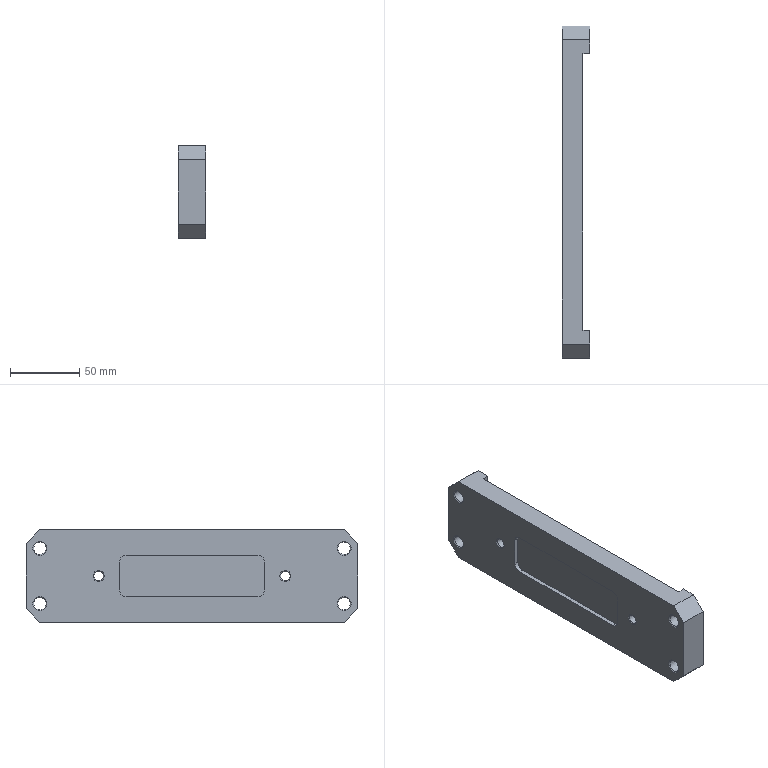Part | NX | features DATUM_CSYS 6, SIMPLE HOLE 6, SKETCH 5, EXTRUDE 3, HOLE PACKAGE 2, LINKED_CURVE 2, SYMBOLIC_THREAD 2, BLEND 1, CHAMFER 1, LINKED_FACE 1 | 1 solid | 41 faces | box 20 x 240 x 67 mm | volume 234977 mm3 | plane 19 | cone 12 | cylinder 10 | commonest cylinder face diameters 9 x4 10 x4 6.8 x2
STEP:
#1=CARTESIAN_POINT('',(65.,-120.,-393.));
#2=VERTEX_POINT('',#1);
#3=CARTESIAN_POINT('',(65.,-120.,-440.));
#4=VERTEX_POINT('',#3);
#5=CARTESIAN_POINT('',(65.,-120.,-383.));
#6=DIRECTION('',(0.,0.,-1.));
#7=VECTOR('',#6,1000.);
#8=LINE('',#5,#7);
#9=EDGE_CURVE('',#2,#4,#8,.T.);
#10=ORIENTED_EDGE('',*,*,#9,.F.);
#11=CARTESIAN_POINT('',(65.,-110.,-383.));
#12=VERTEX_POINT('',#11);
#13=CARTESIAN_POINT('',(65.,-120.,-393.));
#14=DIRECTION('',(0.,-0.7071,-0.7071));
#15=VECTOR('',#14,1000.);
#16=LINE('',#13,#15);
#17=EDGE_CURVE('',#2,#12,#16,.F.);
#18=ORIENTED_EDGE('',*,*,#17,.T.);
#19=CARTESIAN_POINT('',(65.,110.,-383.));
#20=VERTEX_POINT('',#19);
#21=CARTESIAN_POINT('',(65.,120.,-383.));
#22=DIRECTION('',(0.,-1.,0.));
#23=VECTOR('',#22,1000.);
#24=LINE('',#21,#23);
#25=EDGE_CURVE('',#20,#12,#24,.T.);
#26=ORIENTED_EDGE('',*,*,#25,.F.);
#27=CARTESIAN_POINT('',(65.,120.,-393.));
#28=VERTEX_POINT('',#27);
#29=CARTESIAN_POINT('',(65.,110.,-383.));
#30=DIRECTION('',(0.,-0.7071,0.7071));
#31=VECTOR('',#30,1000.);
#32=LINE('',#29,#31);
#33=EDGE_CURVE('',#20,#28,#32,.F.);
#34=ORIENTED_EDGE('',*,*,#33,.T.);
#35=CARTESIAN_POINT('',(65.,120.,-440.));
#36=VERTEX_POINT('',#35);
#37=CARTESIAN_POINT('',(65.,120.,-450.));
#38=DIRECTION('',(0.,0.,1.));
#39=VECTOR('',#38,1000.);
#40=LINE('',#37,#39);
#41=EDGE_CURVE('',#36,#28,#40,.T.);
#42=ORIENTED_EDGE('',*,*,#41,.F.);
#43=CARTESIAN_POINT('',(65.,110.,-450.));
#44=VERTEX_POINT('',#43);
#45=CARTESIAN_POINT('',(65.,120.,-440.));
#46=DIRECTION('',(0.,0.7071,0.7071));
#47=VECTOR('',#46,1000.);
#48=LINE('',#45,#47);
#49=EDGE_CURVE('',#36,#44,#48,.F.);
#50=ORIENTED_EDGE('',*,*,#49,.T.);
#51=CARTESIAN_POINT('',(65.,-110.,-450.));
#52=VERTEX_POINT('',#51);
#53=CARTESIAN_POINT('',(65.,-120.,-450.));
#54=DIRECTION('',(0.,1.,0.));
#55=VECTOR('',#54,1000.);
#56=LINE('',#53,#55);
#57=EDGE_CURVE('',#52,#44,#56,.T.);
#58=ORIENTED_EDGE('',*,*,#57,.F.);
#59=CARTESIAN_POINT('',(65.,-110.,-450.));
#60=DIRECTION('',(0.,0.7071,-0.7071));
#61=VECTOR('',#60,1000.);
#62=LINE('',#59,#61);
#63=EDGE_CURVE('',#52,#4,#62,.F.);
#64=ORIENTED_EDGE('',*,*,#63,.T.);
#65=EDGE_LOOP('',(#10,#18,#26,#34,#42,#50,#58,#64));
#66=FACE_BOUND('',#65,.T.);
#67=CARTESIAN_POINT('',(65.,-67.5,-420.5));
#68=VERTEX_POINT('',#67);
#69=CARTESIAN_POINT('',(65.,-67.5,-416.5));
#70=DIRECTION('',(1.,0.,0.));
#71=DIRECTION('',(0.,0.,-1.));
#72=AXIS2_PLACEMENT_3D('',#69,#70,#71);
#73=CIRCLE('',#72,4.);
#74=EDGE_CURVE('',#68,#68,#73,.T.);
#75=ORIENTED_EDGE('',*,*,#74,.T.);
#76=EDGE_LOOP('',(#75));
#77=FACE_BOUND('',#76,.T.);
#78=CARTESIAN_POINT('',(65.,67.5,-420.5));
#79=VERTEX_POINT('',#78);
#80=CARTESIAN_POINT('',(65.,67.5,-416.5));
#81=DIRECTION('',(1.,0.,0.));
#82=DIRECTION('',(0.,0.,-1.));
#83=AXIS2_PLACEMENT_3D('',#80,#81,#82);
#84=CIRCLE('',#83,4.);
#85=EDGE_CURVE('',#79,#79,#84,.T.);
#86=ORIENTED_EDGE('',*,*,#85,.T.);
#87=EDGE_LOOP('',(#86));
#88=FACE_BOUND('',#87,.T.);
#89=CARTESIAN_POINT('',(65.,110.,-401.6));
#90=VERTEX_POINT('',#89);
#91=CARTESIAN_POINT('',(65.,110.,-396.5));
#92=DIRECTION('',(1.,0.,0.));
#93=DIRECTION('',(0.,0.,-1.));
#94=AXIS2_PLACEMENT_3D('',#91,#92,#93);
#95=CIRCLE('',#94,5.1);
#96=EDGE_CURVE('',#90,#90,#95,.T.);
#97=ORIENTED_EDGE('',*,*,#96,.T.);
#98=EDGE_LOOP('',(#97));
#99=FACE_BOUND('',#98,.T.);
#100=CARTESIAN_POINT('',(65.,110.,-441.6));
#101=VERTEX_POINT('',#100);
#102=CARTESIAN_POINT('',(65.,110.,-436.5));
#103=DIRECTION('',(1.,0.,0.));
#104=DIRECTION('',(0.,0.,-1.));
#105=AXIS2_PLACEMENT_3D('',#102,#103,#104);
#106=CIRCLE('',#105,5.1);
#107=EDGE_CURVE('',#101,#101,#106,.T.);
#108=ORIENTED_EDGE('',*,*,#107,.T.);
#109=EDGE_LOOP('',(#108));
#110=FACE_BOUND('',#109,.T.);
#111=CARTESIAN_POINT('',(65.,-110.,-401.6));
#112=VERTEX_POINT('',#111);
#113=CARTESIAN_POINT('',(65.,-110.,-396.5));
#114=DIRECTION('',(1.,0.,0.));
#115=DIRECTION('',(0.,0.,-1.));
#116=AXIS2_PLACEMENT_3D('',#113,#114,#115);
#117=CIRCLE('',#116,5.1);
#118=EDGE_CURVE('',#112,#112,#117,.T.);
#119=ORIENTED_EDGE('',*,*,#118,.T.);
#120=EDGE_LOOP('',(#119));
#121=FACE_BOUND('',#120,.T.);
#122=CARTESIAN_POINT('',(65.,-110.,-441.6));
#123=VERTEX_POINT('',#122);
#124=CARTESIAN_POINT('',(65.,-110.,-436.5));
#125=DIRECTION('',(1.,0.,0.));
#126=DIRECTION('',(0.,0.,-1.));
#127=AXIS2_PLACEMENT_3D('',#124,#125,#126);
#128=CIRCLE('',#127,5.1);
#129=EDGE_CURVE('',#123,#123,#128,.T.);
#130=ORIENTED_EDGE('',*,*,#129,.T.);
#131=EDGE_LOOP('',(#130));
#132=FACE_BOUND('',#131,.T.);
#133=CARTESIAN_POINT('',(65.,-52.5,-426.5));
#134=VERTEX_POINT('',#133);
#135=CARTESIAN_POINT('',(65.,-52.5,-406.5));
#136=VERTEX_POINT('',#135);
#137=CARTESIAN_POINT('',(65.,-52.5,-431.5));
#138=DIRECTION('',(0.,0.,1.));
#139=VECTOR('',#138,1000.);
#140=LINE('',#137,#139);
#141=EDGE_CURVE('',#134,#136,#140,.T.);
#142=ORIENTED_EDGE('',*,*,#141,.F.);
#143=CARTESIAN_POINT('',(65.,-47.5,-431.5));
#144=VERTEX_POINT('',#143);
#145=CARTESIAN_POINT('',(65.,-47.5,-426.5));
#146=DIRECTION('',(1.,0.,0.));
#147=DIRECTION('',(0.,0.,-1.));
#148=AXIS2_PLACEMENT_3D('',#145,#146,#147);
#149=CIRCLE('',#148,5.);
#150=EDGE_CURVE('',#134,#144,#149,.T.);
#151=ORIENTED_EDGE('',*,*,#150,.T.);
#152=CARTESIAN_POINT('',(65.,47.5,-431.5));
#153=VERTEX_POINT('',#152);
#154=CARTESIAN_POINT('',(65.,52.5,-431.5));
#155=DIRECTION('',(0.,-1.,0.));
#156=VECTOR('',#155,1000.);
#157=LINE('',#154,#156);
#158=EDGE_CURVE('',#153,#144,#157,.T.);
#159=ORIENTED_EDGE('',*,*,#158,.F.);
#160=CARTESIAN_POINT('',(65.,52.5,-426.5));
#161=VERTEX_POINT('',#160);
#162=CARTESIAN_POINT('',(65.,47.5,-426.5));
#163=DIRECTION('',(1.,0.,0.));
#164=DIRECTION('',(0.,0.,-1.));
#165=AXIS2_PLACEMENT_3D('',#162,#163,#164);
#166=CIRCLE('',#165,5.);
#167=EDGE_CURVE('',#153,#161,#166,.T.);
#168=ORIENTED_EDGE('',*,*,#167,.T.);
#169=CARTESIAN_POINT('',(65.,52.5,-406.5));
#170=VERTEX_POINT('',#169);
#171=CARTESIAN_POINT('',(65.,52.5,-401.5));
#172=DIRECTION('',(0.,0.,-1.));
#173=VECTOR('',#172,1000.);
#174=LINE('',#171,#173);
#175=EDGE_CURVE('',#170,#161,#174,.T.);
#176=ORIENTED_EDGE('',*,*,#175,.F.);
#177=CARTESIAN_POINT('',(65.,47.5,-401.5));
#178=VERTEX_POINT('',#177);
#179=CARTESIAN_POINT('',(65.,47.5,-406.5));
#180=DIRECTION('',(1.,0.,0.));
#181=DIRECTION('',(0.,0.,-1.));
#182=AXIS2_PLACEMENT_3D('',#179,#180,#181);
#183=CIRCLE('',#182,5.);
#184=EDGE_CURVE('',#170,#178,#183,.T.);
#185=ORIENTED_EDGE('',*,*,#184,.T.);
#186=CARTESIAN_POINT('',(65.,-47.5,-401.5));
#187=VERTEX_POINT('',#186);
#188=CARTESIAN_POINT('',(65.,-52.5,-401.5));
#189=DIRECTION('',(0.,1.,0.));
#190=VECTOR('',#189,1000.);
#191=LINE('',#188,#190);
#192=EDGE_CURVE('',#187,#178,#191,.T.);
#193=ORIENTED_EDGE('',*,*,#192,.F.);
#194=CARTESIAN_POINT('',(65.,-47.5,-406.5));
#195=DIRECTION('',(1.,0.,0.));
#196=DIRECTION('',(0.,0.,-1.));
#197=AXIS2_PLACEMENT_3D('',#194,#195,#196);
#198=CIRCLE('',#197,5.);
#199=EDGE_CURVE('',#187,#136,#198,.T.);
#200=ORIENTED_EDGE('',*,*,#199,.T.);
#201=EDGE_LOOP('',(#142,#151,#159,#168,#176,#185,#193,#200));
#202=FACE_BOUND('',#201,.T.);
#203=CARTESIAN_POINT('',(65.,0.,0.));
#204=DIRECTION('',(1.,0.,0.));
#205=DIRECTION('',(0.,0.,-1.));
#206=AXIS2_PLACEMENT_3D('',#203,#204,#205);
#207=PLANE('',#206);
#208=ADVANCED_FACE('',(#66,#77,#88,#99,#110,#121,#132,#202),#207,.F.);
#209=CARTESIAN_POINT('',(85.,-110.,-450.));
#210=VERTEX_POINT('',#209);
#211=CARTESIAN_POINT('',(85.,-100.,-450.));
#212=VERTEX_POINT('',#211);
#213=CARTESIAN_POINT('',(85.,-120.,-450.));
#214=DIRECTION('',(0.,1.,0.));
#215=VECTOR('',#214,1000.);
#216=LINE('',#213,#215);
#217=EDGE_CURVE('',#210,#212,#216,.T.);
#218=ORIENTED_EDGE('',*,*,#217,.F.);
#219=CARTESIAN_POINT('',(85.,-110.,-450.));
#220=DIRECTION('',(-1.,0.,0.));
#221=VECTOR('',#220,1000.);
#222=LINE('',#219,#221);
#223=EDGE_CURVE('',#210,#52,#222,.T.);
#224=ORIENTED_EDGE('',*,*,#223,.T.);
#225=ORIENTED_EDGE('',*,*,#57,.T.);
#226=CARTESIAN_POINT('',(85.,110.,-450.));
#227=VERTEX_POINT('',#226);
#228=CARTESIAN_POINT('',(85.,110.,-450.));
#229=DIRECTION('',(1.,0.,0.));
#230=VECTOR('',#229,1000.);
#231=LINE('',#228,#230);
#232=EDGE_CURVE('',#44,#227,#231,.T.);
#233=ORIENTED_EDGE('',*,*,#232,.T.);
#234=CARTESIAN_POINT('',(85.,100.,-450.));
#235=VERTEX_POINT('',#234);
#236=CARTESIAN_POINT('',(85.,-120.,-450.));
#237=DIRECTION('',(0.,1.,0.));
#238=VECTOR('',#237,1000.);
#239=LINE('',#236,#238);
#240=EDGE_CURVE('',#235,#227,#239,.T.);
#241=ORIENTED_EDGE('',*,*,#240,.F.);
#242=CARTESIAN_POINT('',(80.,100.,-450.));
#243=VERTEX_POINT('',#242);
#244=CARTESIAN_POINT('',(80.,100.,-450.));
#245=DIRECTION('',(1.,0.,0.));
#246=VECTOR('',#245,1000.);
#247=LINE('',#244,#246);
#248=EDGE_CURVE('',#243,#235,#247,.T.);
#249=ORIENTED_EDGE('',*,*,#248,.F.);
#250=CARTESIAN_POINT('',(80.,-100.,-450.));
#251=VERTEX_POINT('',#250);
#252=CARTESIAN_POINT('',(80.,-100.,-450.));
#253=DIRECTION('',(0.,1.,0.));
#254=VECTOR('',#253,1000.);
#255=LINE('',#252,#254);
#256=EDGE_CURVE('',#251,#243,#255,.T.);
#257=ORIENTED_EDGE('',*,*,#256,.F.);
#258=CARTESIAN_POINT('',(119.,-100.,-450.));
#259=DIRECTION('',(-1.,0.,0.));
#260=VECTOR('',#259,1000.);
#261=LINE('',#258,#260);
#262=EDGE_CURVE('',#212,#251,#261,.T.);
#263=ORIENTED_EDGE('',*,*,#262,.F.);
#264=EDGE_LOOP('',(#218,#224,#225,#233,#241,#249,#257,#263));
#265=FACE_BOUND('',#264,.T.);
#266=CARTESIAN_POINT('',(85.,-120.,-450.));
#267=DIRECTION('',(0.,0.,1.));
#268=DIRECTION('',(0.,-1.,0.));
#269=AXIS2_PLACEMENT_3D('',#266,#267,#268);
#270=PLANE('',#269);
#271=ADVANCED_FACE('',(#265),#270,.F.);
#272=CARTESIAN_POINT('',(85.,110.,-441.6));
#273=VERTEX_POINT('',#272);
#274=CARTESIAN_POINT('',(85.,110.,-436.5));
#275=DIRECTION('',(1.,0.,0.));
#276=DIRECTION('',(0.,0.,-1.));
#277=AXIS2_PLACEMENT_3D('',#274,#275,#276);
#278=CIRCLE('',#277,5.1);
#279=EDGE_CURVE('',#273,#273,#278,.F.);
#280=ORIENTED_EDGE('',*,*,#279,.T.);
#281=EDGE_LOOP('',(#280));
#282=FACE_BOUND('',#281,.T.);
#283=CARTESIAN_POINT('',(85.,110.,-401.6));
#284=VERTEX_POINT('',#283);
#285=CARTESIAN_POINT('',(85.,110.,-396.5));
#286=DIRECTION('',(1.,0.,0.));
#287=DIRECTION('',(0.,0.,-1.));
#288=AXIS2_PLACEMENT_3D('',#285,#286,#287);
#289=CIRCLE('',#288,5.1);
#290=EDGE_CURVE('',#284,#284,#289,.F.);
#291=ORIENTED_EDGE('',*,*,#290,.T.);
#292=EDGE_LOOP('',(#291));
#293=FACE_BOUND('',#292,.T.);
#294=CARTESIAN_POINT('',(85.,120.,-440.));
#295=VERTEX_POINT('',#294);
#296=CARTESIAN_POINT('',(85.,120.,-393.));
#297=VERTEX_POINT('',#296);
#298=CARTESIAN_POINT('',(85.,120.,-450.));
#299=DIRECTION('',(0.,0.,1.));
#300=VECTOR('',#299,1000.);
#301=LINE('',#298,#300);
#302=EDGE_CURVE('',#295,#297,#301,.T.);
#303=ORIENTED_EDGE('',*,*,#302,.T.);
#304=CARTESIAN_POINT('',(85.,110.,-383.));
#305=VERTEX_POINT('',#304);
#306=CARTESIAN_POINT('',(85.,-136.5,-136.5));
#307=DIRECTION('',(0.,0.7071,-0.7071));
#308=VECTOR('',#307,1000.);
#309=LINE('',#306,#308);
#310=EDGE_CURVE('',#297,#305,#309,.F.);
#311=ORIENTED_EDGE('',*,*,#310,.T.);
#312=CARTESIAN_POINT('',(85.,100.,-383.));
#313=VERTEX_POINT('',#312);
#314=CARTESIAN_POINT('',(85.,120.,-383.));
#315=DIRECTION('',(0.,-1.,0.));
#316=VECTOR('',#315,1000.);
#317=LINE('',#314,#316);
#318=EDGE_CURVE('',#305,#313,#317,.T.);
#319=ORIENTED_EDGE('',*,*,#318,.T.);
#320=CARTESIAN_POINT('',(85.,100.,0.));
#321=DIRECTION('',(0.,0.,1.));
#322=VECTOR('',#321,1000.);
#323=LINE('',#320,#322);
#324=EDGE_CURVE('',#235,#313,#323,.T.);
#325=ORIENTED_EDGE('',*,*,#324,.F.);
#326=ORIENTED_EDGE('',*,*,#240,.T.);
#327=CARTESIAN_POINT('',(85.,280.,-280.));
#328=DIRECTION('',(0.,-0.7071,-0.7071));
#329=VECTOR('',#328,1000.);
#330=LINE('',#327,#329);
#331=EDGE_CURVE('',#227,#295,#330,.F.);
#332=ORIENTED_EDGE('',*,*,#331,.T.);
#333=EDGE_LOOP('',(#303,#311,#319,#325,#326,#332));
#334=FACE_BOUND('',#333,.T.);
#335=CARTESIAN_POINT('',(85.,0.,0.));
#336=DIRECTION('',(1.,0.,0.));
#337=DIRECTION('',(0.,0.,-1.));
#338=AXIS2_PLACEMENT_3D('',#335,#336,#337);
#339=PLANE('',#338);
#340=ADVANCED_FACE('',(#282,#293,#334),#339,.T.);
#341=CARTESIAN_POINT('',(85.,-120.,-393.));
#342=VERTEX_POINT('',#341);
#343=CARTESIAN_POINT('',(85.,-120.,-440.));
#344=VERTEX_POINT('',#343);
#345=CARTESIAN_POINT('',(85.,-120.,-383.));
#346=DIRECTION('',(0.,0.,-1.));
#347=VECTOR('',#346,1000.);
#348=LINE('',#345,#347);
#349=EDGE_CURVE('',#342,#344,#348,.T.);
#350=ORIENTED_EDGE('',*,*,#349,.F.);
#351=CARTESIAN_POINT('',(85.,-120.,-393.));
#352=DIRECTION('',(-1.,0.,0.));
#353=VECTOR('',#352,1000.);
#354=LINE('',#351,#353);
#355=EDGE_CURVE('',#342,#2,#354,.T.);
#356=ORIENTED_EDGE('',*,*,#355,.T.);
#357=ORIENTED_EDGE('',*,*,#9,.T.);
#358=CARTESIAN_POINT('',(85.,-120.,-440.));
#359=DIRECTION('',(1.,0.,0.));
#360=VECTOR('',#359,1000.);
#361=LINE('',#358,#360);
#362=EDGE_CURVE('',#4,#344,#361,.T.);
#363=ORIENTED_EDGE('',*,*,#362,.T.);
#364=EDGE_LOOP('',(#350,#356,#357,#363));
#365=FACE_BOUND('',#364,.T.);
#366=CARTESIAN_POINT('',(85.,-120.,-383.));
#367=DIRECTION('',(0.,1.,0.));
#368=DIRECTION('',(0.,0.,1.));
#369=AXIS2_PLACEMENT_3D('',#366,#367,#368);
#370=PLANE('',#369);
#371=ADVANCED_FACE('',(#365),#370,.F.);
#372=ORIENTED_EDGE('',*,*,#41,.T.);
#373=CARTESIAN_POINT('',(85.,120.,-393.));
#374=DIRECTION('',(1.,0.,0.));
#375=VECTOR('',#374,1000.);
#376=LINE('',#373,#375);
#377=EDGE_CURVE('',#28,#297,#376,.T.);
#378=ORIENTED_EDGE('',*,*,#377,.T.);
#379=ORIENTED_EDGE('',*,*,#302,.F.);
#380=CARTESIAN_POINT('',(85.,120.,-440.));
#381=DIRECTION('',(-1.,0.,0.));
#382=VECTOR('',#381,1000.);
#383=LINE('',#380,#382);
#384=EDGE_CURVE('',#295,#36,#383,.T.);
#385=ORIENTED_EDGE('',*,*,#384,.T.);
#386=EDGE_LOOP('',(#372,#378,#379,#385));
#387=FACE_BOUND('',#386,.T.);
#388=CARTESIAN_POINT('',(85.,120.,-450.));
#389=DIRECTION('',(0.,-1.,0.));
#390=DIRECTION('',(0.,0.,-1.));
#391=AXIS2_PLACEMENT_3D('',#388,#389,#390);
#392=PLANE('',#391);
#393=ADVANCED_FACE('',(#387),#392,.F.);
#394=ORIENTED_EDGE('',*,*,#25,.T.);
#395=CARTESIAN_POINT('',(85.,-110.,-383.));
#396=VERTEX_POINT('',#395);
#397=CARTESIAN_POINT('',(85.,-110.,-383.));
#398=DIRECTION('',(1.,0.,0.));
#399=VECTOR('',#398,1000.);
#400=LINE('',#397,#399);
#401=EDGE_CURVE('',#12,#396,#400,.T.);
#402=ORIENTED_EDGE('',*,*,#401,.T.);
#403=CARTESIAN_POINT('',(85.,-100.,-383.));
#404=VERTEX_POINT('',#403);
#405=CARTESIAN_POINT('',(85.,120.,-383.));
#406=DIRECTION('',(0.,-1.,0.));
#407=VECTOR('',#406,1000.);
#408=LINE('',#405,#407);
#409=EDGE_CURVE('',#404,#396,#408,.T.);
#410=ORIENTED_EDGE('',*,*,#409,.F.);
#411=CARTESIAN_POINT('',(80.,-100.,-383.));
#412=VERTEX_POINT('',#411);
#413=CARTESIAN_POINT('',(85.,-100.,-383.));
#414=DIRECTION('',(-1.,0.,0.));
#415=VECTOR('',#414,1000.);
#416=LINE('',#413,#415);
#417=EDGE_CURVE('',#404,#412,#416,.T.);
#418=ORIENTED_EDGE('',*,*,#417,.T.);
#419=CARTESIAN_POINT('',(80.,100.,-383.));
#420=VERTEX_POINT('',#419);
#421=CARTESIAN_POINT('',(80.,120.,-383.));
#422=DIRECTION('',(0.,1.,0.));
#423=VECTOR('',#422,1000.);
#424=LINE('',#421,#423);
#425=EDGE_CURVE('',#412,#420,#424,.T.);
#426=ORIENTED_EDGE('',*,*,#425,.T.);
#427=CARTESIAN_POINT('',(85.,100.,-383.));
#428=DIRECTION('',(1.,0.,0.));
#429=VECTOR('',#428,1000.);
#430=LINE('',#427,#429);
#431=EDGE_CURVE('',#420,#313,#430,.T.);
#432=ORIENTED_EDGE('',*,*,#431,.T.);
#433=ORIENTED_EDGE('',*,*,#318,.F.);
#434=CARTESIAN_POINT('',(85.,110.,-383.));
#435=DIRECTION('',(-1.,0.,0.));
#436=VECTOR('',#435,1000.);
#437=LINE('',#434,#436);
#438=EDGE_CURVE('',#305,#20,#437,.T.);
#439=ORIENTED_EDGE('',*,*,#438,.T.);
#440=EDGE_LOOP('',(#394,#402,#410,#418,#426,#432,#433,#439));
#441=FACE_BOUND('',#440,.T.);
#442=CARTESIAN_POINT('',(85.,120.,-383.));
#443=DIRECTION('',(0.,0.,-1.));
#444=DIRECTION('',(-1.,0.,0.));
#445=AXIS2_PLACEMENT_3D('',#442,#443,#444);
#446=PLANE('',#445);
#447=ADVANCED_FACE('',(#441),#446,.F.);
#448=CARTESIAN_POINT('',(85.,-110.,-441.6));
#449=VERTEX_POINT('',#448);
#450=CARTESIAN_POINT('',(85.,-110.,-436.5));
#451=DIRECTION('',(1.,0.,0.));
#452=DIRECTION('',(0.,0.,-1.));
#453=AXIS2_PLACEMENT_3D('',#450,#451,#452);
#454=CIRCLE('',#453,5.1);
#455=EDGE_CURVE('',#449,#449,#454,.F.);
#456=ORIENTED_EDGE('',*,*,#455,.T.);
#457=EDGE_LOOP('',(#456));
#458=FACE_BOUND('',#457,.T.);
#459=CARTESIAN_POINT('',(85.,-110.,-401.6));
#460=VERTEX_POINT('',#459);
#461=CARTESIAN_POINT('',(85.,-110.,-396.5));
#462=DIRECTION('',(1.,0.,0.));
#463=DIRECTION('',(0.,0.,-1.));
#464=AXIS2_PLACEMENT_3D('',#461,#462,#463);
#465=CIRCLE('',#464,5.1);
#466=EDGE_CURVE('',#460,#460,#465,.F.);
#467=ORIENTED_EDGE('',*,*,#466,.T.);
#468=EDGE_LOOP('',(#467));
#469=FACE_BOUND('',#468,.T.);
#470=ORIENTED_EDGE('',*,*,#409,.T.);
#471=CARTESIAN_POINT('',(85.,136.5,-136.5));
#472=DIRECTION('',(0.,0.7071,0.7071));
#473=VECTOR('',#472,1000.);
#474=LINE('',#471,#473);
#475=EDGE_CURVE('',#396,#342,#474,.F.);
#476=ORIENTED_EDGE('',*,*,#475,.T.);
#477=ORIENTED_EDGE('',*,*,#349,.T.);
#478=CARTESIAN_POINT('',(85.,-280.,-280.));
#479=DIRECTION('',(0.,-0.7071,0.7071));
#480=VECTOR('',#479,1000.);
#481=LINE('',#478,#480);
#482=EDGE_CURVE('',#344,#210,#481,.F.);
#483=ORIENTED_EDGE('',*,*,#482,.T.);
#484=ORIENTED_EDGE('',*,*,#217,.T.);
#485=CARTESIAN_POINT('',(85.,-100.,0.));
#486=DIRECTION('',(0.,0.,-1.));
#487=VECTOR('',#486,1000.);
#488=LINE('',#485,#487);
#489=EDGE_CURVE('',#404,#212,#488,.T.);
#490=ORIENTED_EDGE('',*,*,#489,.F.);
#491=EDGE_LOOP('',(#470,#476,#477,#483,#484,#490));
#492=FACE_BOUND('',#491,.T.);
#493=CARTESIAN_POINT('',(85.,0.,0.));
#494=DIRECTION('',(1.,0.,0.));
#495=DIRECTION('',(0.,0.,-1.));
#496=AXIS2_PLACEMENT_3D('',#493,#494,#495);
#497=PLANE('',#496);
#498=ADVANCED_FACE('',(#458,#469,#492),#497,.T.);
#499=CARTESIAN_POINT('',(80.,63.5,-416.5));
#500=VERTEX_POINT('',#499);
#501=CARTESIAN_POINT('',(80.,67.5,-416.5));
#502=DIRECTION('',(-1.,0.,0.));
#503=DIRECTION('',(0.,-1.,0.));
#504=AXIS2_PLACEMENT_3D('',#501,#502,#503);
#505=CIRCLE('',#504,4.);
#506=EDGE_CURVE('',#500,#500,#505,.T.);
#507=ORIENTED_EDGE('',*,*,#506,.T.);
#508=EDGE_LOOP('',(#507));
#509=FACE_BOUND('',#508,.T.);
#510=CARTESIAN_POINT('',(80.,-71.5,-416.5));
#511=VERTEX_POINT('',#510);
#512=CARTESIAN_POINT('',(80.,-67.5,-416.5));
#513=DIRECTION('',(-1.,0.,0.));
#514=DIRECTION('',(0.,-1.,0.));
#515=AXIS2_PLACEMENT_3D('',#512,#513,#514);
#516=CIRCLE('',#515,4.);
#517=EDGE_CURVE('',#511,#511,#516,.T.);
#518=ORIENTED_EDGE('',*,*,#517,.T.);
#519=EDGE_LOOP('',(#518));
#520=FACE_BOUND('',#519,.T.);
#521=CARTESIAN_POINT('',(80.,-100.,-255.));
#522=DIRECTION('',(0.,0.,-1.));
#523=VECTOR('',#522,1000.);
#524=LINE('',#521,#523);
#525=EDGE_CURVE('',#251,#412,#524,.F.);
#526=ORIENTED_EDGE('',*,*,#525,.F.);
#527=ORIENTED_EDGE('',*,*,#256,.T.);
#528=CARTESIAN_POINT('',(80.,100.,-255.));
#529=DIRECTION('',(0.,0.,-1.));
#530=VECTOR('',#529,1000.);
#531=LINE('',#528,#530);
#532=EDGE_CURVE('',#243,#420,#531,.F.);
#533=ORIENTED_EDGE('',*,*,#532,.T.);
#534=ORIENTED_EDGE('',*,*,#425,.F.);
#535=EDGE_LOOP('',(#526,#527,#533,#534));
#536=FACE_BOUND('',#535,.T.);
#537=CARTESIAN_POINT('',(80.,-100.,-255.));
#538=DIRECTION('',(-1.,0.,0.));
#539=DIRECTION('',(0.,-1.,0.));
#540=AXIS2_PLACEMENT_3D('',#537,#538,#539);
#541=PLANE('',#540);
#542=ADVANCED_FACE('',(#509,#520,#536),#541,.F.);
#543=ORIENTED_EDGE('',*,*,#532,.F.);
#544=ORIENTED_EDGE('',*,*,#248,.T.);
#545=ORIENTED_EDGE('',*,*,#324,.T.);
#546=ORIENTED_EDGE('',*,*,#431,.F.);
#547=EDGE_LOOP('',(#543,#544,#545,#546));
#548=FACE_BOUND('',#547,.T.);
#549=CARTESIAN_POINT('',(80.,100.,-255.));
#550=DIRECTION('',(0.,1.,0.));
#551=DIRECTION('',(0.,0.,1.));
#552=AXIS2_PLACEMENT_3D('',#549,#550,#551);
#553=PLANE('',#552);
#554=ADVANCED_FACE('',(#548),#553,.F.);
#555=ORIENTED_EDGE('',*,*,#489,.T.);
#556=ORIENTED_EDGE('',*,*,#262,.T.);
#557=ORIENTED_EDGE('',*,*,#525,.T.);
#558=ORIENTED_EDGE('',*,*,#417,.F.);
#559=EDGE_LOOP('',(#555,#556,#557,#558));
#560=FACE_BOUND('',#559,.T.);
#561=CARTESIAN_POINT('',(119.,-100.,-255.));
#562=DIRECTION('',(0.,-1.,0.));
#563=DIRECTION('',(0.,0.,-1.));
#564=AXIS2_PLACEMENT_3D('',#561,#562,#563);
#565=PLANE('',#564);
#566=ADVANCED_FACE('',(#560),#565,.F.);
#567=ORIENTED_EDGE('',*,*,#475,.F.);
#568=ORIENTED_EDGE('',*,*,#401,.F.);
#569=ORIENTED_EDGE('',*,*,#17,.F.);
#570=ORIENTED_EDGE('',*,*,#355,.F.);
#571=EDGE_LOOP('',(#567,#568,#569,#570));
#572=FACE_BOUND('',#571,.T.);
#573=CARTESIAN_POINT('',(85.,-120.,-393.));
#574=DIRECTION('',(0.,0.7071,-0.7071));
#575=DIRECTION('',(-1.,0.,0.));
#576=AXIS2_PLACEMENT_3D('',#573,#574,#575);
#577=PLANE('',#576);
#578=ADVANCED_FACE('',(#572),#577,.F.);
#579=ORIENTED_EDGE('',*,*,#482,.F.);
#580=ORIENTED_EDGE('',*,*,#362,.F.);
#581=ORIENTED_EDGE('',*,*,#63,.F.);
#582=ORIENTED_EDGE('',*,*,#223,.F.);
#583=EDGE_LOOP('',(#579,#580,#581,#582));
#584=FACE_BOUND('',#583,.T.);
#585=CARTESIAN_POINT('',(85.,-110.,-450.));
#586=DIRECTION('',(0.,0.7071,0.7071));
#587=DIRECTION('',(-1.,0.,0.));
#588=AXIS2_PLACEMENT_3D('',#585,#586,#587);
#589=PLANE('',#588);
#590=ADVANCED_FACE('',(#584),#589,.F.);
#591=ORIENTED_EDGE('',*,*,#310,.F.);
#592=ORIENTED_EDGE('',*,*,#377,.F.);
#593=ORIENTED_EDGE('',*,*,#33,.F.);
#594=ORIENTED_EDGE('',*,*,#438,.F.);
#595=EDGE_LOOP('',(#591,#592,#593,#594));
#596=FACE_BOUND('',#595,.T.);
#597=CARTESIAN_POINT('',(85.,110.,-383.));
#598=DIRECTION('',(0.,-0.7071,-0.7071));
#599=DIRECTION('',(-1.,0.,0.));
#600=AXIS2_PLACEMENT_3D('',#597,#598,#599);
#601=PLANE('',#600);
#602=ADVANCED_FACE('',(#596),#601,.F.);
#603=ORIENTED_EDGE('',*,*,#331,.F.);
#604=ORIENTED_EDGE('',*,*,#232,.F.);
#605=ORIENTED_EDGE('',*,*,#49,.F.);
#606=ORIENTED_EDGE('',*,*,#384,.F.);
#607=EDGE_LOOP('',(#603,#604,#605,#606));
#608=FACE_BOUND('',#607,.T.);
#609=CARTESIAN_POINT('',(85.,120.,-440.));
#610=DIRECTION('',(0.,-0.7071,0.7071));
#611=DIRECTION('',(-1.,0.,0.));
#612=AXIS2_PLACEMENT_3D('',#609,#610,#611);
#613=PLANE('',#612);
#614=ADVANCED_FACE('',(#608),#613,.F.);
#615=CARTESIAN_POINT('',(79.4,-67.5,-413.1));
#616=VERTEX_POINT('',#615);
#617=CARTESIAN_POINT('',(79.4,-67.5,-416.5));
#618=DIRECTION('',(-1.,0.,0.));
#619=DIRECTION('',(0.,0.,1.));
#620=AXIS2_PLACEMENT_3D('',#617,#618,#619);
#621=CIRCLE('',#620,3.4);
#622=EDGE_CURVE('',#616,#616,#621,.F.);
#623=ORIENTED_EDGE('',*,*,#622,.T.);
#624=EDGE_LOOP('',(#623));
#625=FACE_BOUND('',#624,.T.);
#626=CARTESIAN_POINT('',(65.6,-67.5,-419.9));
#627=VERTEX_POINT('',#626);
#628=CARTESIAN_POINT('',(65.6,-67.5,-416.5));
#629=DIRECTION('',(1.,0.,0.));
#630=DIRECTION('',(0.,0.,-1.));
#631=AXIS2_PLACEMENT_3D('',#628,#629,#630);
#632=CIRCLE('',#631,3.4);
#633=EDGE_CURVE('',#627,#627,#632,.F.);
#634=ORIENTED_EDGE('',*,*,#633,.T.);
#635=EDGE_LOOP('',(#634));
#636=FACE_BOUND('',#635,.T.);
#637=CARTESIAN_POINT('',(65.,-67.5,-416.5));
#638=DIRECTION('',(1.,0.,0.));
#639=DIRECTION('',(0.,0.,-1.));
#640=AXIS2_PLACEMENT_3D('',#637,#638,#639);
#641=CYLINDRICAL_SURFACE('',#640,3.4);
#642=ADVANCED_FACE('',(#625,#636),#641,.F.);
#643=ORIENTED_EDGE('',*,*,#633,.F.);
#644=EDGE_LOOP('',(#643));
#645=FACE_BOUND('',#644,.T.);
#646=ORIENTED_EDGE('',*,*,#74,.F.);
#647=EDGE_LOOP('',(#646));
#648=FACE_BOUND('',#647,.T.);
#649=CARTESIAN_POINT('',(65.,-67.5,-416.5));
#650=DIRECTION('',(-1.,0.,0.));
#651=DIRECTION('',(0.,0.,1.));
#652=AXIS2_PLACEMENT_3D('',#649,#650,#651);
#653=CONICAL_SURFACE('',#652,4.,0.7854);
#654=ADVANCED_FACE('',(#645,#648),#653,.F.);
#655=ORIENTED_EDGE('',*,*,#622,.F.);
#656=EDGE_LOOP('',(#655));
#657=FACE_BOUND('',#656,.T.);
#658=ORIENTED_EDGE('',*,*,#517,.F.);
#659=EDGE_LOOP('',(#658));
#660=FACE_BOUND('',#659,.T.);
#661=CARTESIAN_POINT('',(80.,-67.5,-416.5));
#662=DIRECTION('',(1.,0.,0.));
#663=DIRECTION('',(0.,0.,-1.));
#664=AXIS2_PLACEMENT_3D('',#661,#662,#663);
#665=CONICAL_SURFACE('',#664,4.,0.7854);
#666=ADVANCED_FACE('',(#657,#660),#665,.F.);
#667=CARTESIAN_POINT('',(79.4,67.5,-413.1));
#668=VERTEX_POINT('',#667);
#669=CARTESIAN_POINT('',(79.4,67.5,-416.5));
#670=DIRECTION('',(-1.,0.,0.));
#671=DIRECTION('',(0.,0.,1.));
#672=AXIS2_PLACEMENT_3D('',#669,#670,#671);
#673=CIRCLE('',#672,3.4);
#674=EDGE_CURVE('',#668,#668,#673,.F.);
#675=ORIENTED_EDGE('',*,*,#674,.T.);
#676=EDGE_LOOP('',(#675));
#677=FACE_BOUND('',#676,.T.);
#678=CARTESIAN_POINT('',(65.6,67.5,-419.9));
#679=VERTEX_POINT('',#678);
#680=CARTESIAN_POINT('',(65.6,67.5,-416.5));
#681=DIRECTION('',(1.,0.,0.));
#682=DIRECTION('',(0.,0.,-1.));
#683=AXIS2_PLACEMENT_3D('',#680,#681,#682);
#684=CIRCLE('',#683,3.4);
#685=EDGE_CURVE('',#679,#679,#684,.F.);
#686=ORIENTED_EDGE('',*,*,#685,.T.);
#687=EDGE_LOOP('',(#686));
#688=FACE_BOUND('',#687,.T.);
#689=CARTESIAN_POINT('',(65.,67.5,-416.5));
#690=DIRECTION('',(1.,0.,0.));
#691=DIRECTION('',(0.,0.,-1.));
#692=AXIS2_PLACEMENT_3D('',#689,#690,#691);
#693=CYLINDRICAL_SURFACE('',#692,3.4);
#694=ADVANCED_FACE('',(#677,#688),#693,.F.);
#695=ORIENTED_EDGE('',*,*,#685,.F.);
#696=EDGE_LOOP('',(#695));
#697=FACE_BOUND('',#696,.T.);
#698=ORIENTED_EDGE('',*,*,#85,.F.);
#699=EDGE_LOOP('',(#698));
#700=FACE_BOUND('',#699,.T.);
#701=CARTESIAN_POINT('',(65.,67.5,-416.5));
#702=DIRECTION('',(-1.,0.,0.));
#703=DIRECTION('',(0.,0.,1.));
#704=AXIS2_PLACEMENT_3D('',#701,#702,#703);
#705=CONICAL_SURFACE('',#704,4.,0.7854);
#706=ADVANCED_FACE('',(#697,#700),#705,.F.);
#707=ORIENTED_EDGE('',*,*,#674,.F.);
#708=EDGE_LOOP('',(#707));
#709=FACE_BOUND('',#708,.T.);
#710=ORIENTED_EDGE('',*,*,#506,.F.);
#711=EDGE_LOOP('',(#710));
#712=FACE_BOUND('',#711,.T.);
#713=CARTESIAN_POINT('',(80.,67.5,-416.5));
#714=DIRECTION('',(1.,0.,0.));
#715=DIRECTION('',(0.,0.,-1.));
#716=AXIS2_PLACEMENT_3D('',#713,#714,#715);
#717=CONICAL_SURFACE('',#716,4.,0.7854);
#718=ADVANCED_FACE('',(#709,#712),#717,.F.);
#719=CARTESIAN_POINT('',(84.4,110.,-401.));
#720=VERTEX_POINT('',#719);
#721=CARTESIAN_POINT('',(84.4,110.,-396.5));
#722=DIRECTION('',(1.,0.,0.));
#723=DIRECTION('',(0.,0.,-1.));
#724=AXIS2_PLACEMENT_3D('',#721,#722,#723);
#725=CIRCLE('',#724,4.5);
#726=EDGE_CURVE('',#720,#720,#725,.T.);
#727=ORIENTED_EDGE('',*,*,#726,.T.);
#728=EDGE_LOOP('',(#727));
#729=FACE_BOUND('',#728,.T.);
#730=CARTESIAN_POINT('',(65.6,110.,-401.));
#731=VERTEX_POINT('',#730);
#732=CARTESIAN_POINT('',(65.6,110.,-396.5));
#733=DIRECTION('',(1.,0.,0.));
#734=DIRECTION('',(0.,0.,-1.));
#735=AXIS2_PLACEMENT_3D('',#732,#733,#734);
#736=CIRCLE('',#735,4.5);
#737=EDGE_CURVE('',#731,#731,#736,.F.);
#738=ORIENTED_EDGE('',*,*,#737,.T.);
#739=EDGE_LOOP('',(#738));
#740=FACE_BOUND('',#739,.T.);
#741=CARTESIAN_POINT('',(65.,110.,-396.5));
#742=DIRECTION('',(1.,0.,0.));
#743=DIRECTION('',(0.,0.,-1.));
#744=AXIS2_PLACEMENT_3D('',#741,#742,#743);
#745=CYLINDRICAL_SURFACE('',#744,4.5);
#746=ADVANCED_FACE('',(#729,#740),#745,.F.);
#747=ORIENTED_EDGE('',*,*,#737,.F.);
#748=EDGE_LOOP('',(#747));
#749=FACE_BOUND('',#748,.T.);
#750=ORIENTED_EDGE('',*,*,#96,.F.);
#751=EDGE_LOOP('',(#750));
#752=FACE_BOUND('',#751,.T.);
#753=CARTESIAN_POINT('',(65.,110.,-396.5));
#754=DIRECTION('',(-1.,0.,0.));
#755=DIRECTION('',(0.,0.,1.));
#756=AXIS2_PLACEMENT_3D('',#753,#754,#755);
#757=CONICAL_SURFACE('',#756,5.1,0.7854);
#758=ADVANCED_FACE('',(#749,#752),#757,.F.);
#759=ORIENTED_EDGE('',*,*,#290,.F.);
#760=EDGE_LOOP('',(#759));
#761=FACE_BOUND('',#760,.T.);
#762=ORIENTED_EDGE('',*,*,#726,.F.);
#763=EDGE_LOOP('',(#762));
#764=FACE_BOUND('',#763,.T.);
#765=CARTESIAN_POINT('',(84.4,110.,-396.5));
#766=DIRECTION('',(1.,0.,0.));
#767=DIRECTION('',(0.,0.,-1.));
#768=AXIS2_PLACEMENT_3D('',#765,#766,#767);
#769=CONICAL_SURFACE('',#768,4.5,0.7854);
#770=ADVANCED_FACE('',(#761,#764),#769,.F.);
#771=CARTESIAN_POINT('',(84.4,110.,-441.));
#772=VERTEX_POINT('',#771);
#773=CARTESIAN_POINT('',(84.4,110.,-436.5));
#774=DIRECTION('',(1.,0.,0.));
#775=DIRECTION('',(0.,0.,-1.));
#776=AXIS2_PLACEMENT_3D('',#773,#774,#775);
#777=CIRCLE('',#776,4.5);
#778=EDGE_CURVE('',#772,#772,#777,.T.);
#779=ORIENTED_EDGE('',*,*,#778,.T.);
#780=EDGE_LOOP('',(#779));
#781=FACE_BOUND('',#780,.T.);
#782=CARTESIAN_POINT('',(65.6,110.,-441.));
#783=VERTEX_POINT('',#782);
#784=CARTESIAN_POINT('',(65.6,110.,-436.5));
#785=DIRECTION('',(1.,0.,0.));
#786=DIRECTION('',(0.,0.,-1.));
#787=AXIS2_PLACEMENT_3D('',#784,#785,#786);
#788=CIRCLE('',#787,4.5);
#789=EDGE_CURVE('',#783,#783,#788,.F.);
#790=ORIENTED_EDGE('',*,*,#789,.T.);
#791=EDGE_LOOP('',(#790));
#792=FACE_BOUND('',#791,.T.);
#793=CARTESIAN_POINT('',(65.,110.,-436.5));
#794=DIRECTION('',(1.,0.,0.));
#795=DIRECTION('',(0.,0.,-1.));
#796=AXIS2_PLACEMENT_3D('',#793,#794,#795);
#797=CYLINDRICAL_SURFACE('',#796,4.5);
#798=ADVANCED_FACE('',(#781,#792),#797,.F.);
#799=ORIENTED_EDGE('',*,*,#789,.F.);
#800=EDGE_LOOP('',(#799));
#801=FACE_BOUND('',#800,.T.);
#802=ORIENTED_EDGE('',*,*,#107,.F.);
#803=EDGE_LOOP('',(#802));
#804=FACE_BOUND('',#803,.T.);
#805=CARTESIAN_POINT('',(65.,110.,-436.5));
#806=DIRECTION('',(-1.,0.,0.));
#807=DIRECTION('',(0.,0.,1.));
#808=AXIS2_PLACEMENT_3D('',#805,#806,#807);
#809=CONICAL_SURFACE('',#808,5.1,0.7854);
#810=ADVANCED_FACE('',(#801,#804),#809,.F.);
#811=ORIENTED_EDGE('',*,*,#279,.F.);
#812=EDGE_LOOP('',(#811));
#813=FACE_BOUND('',#812,.T.);
#814=ORIENTED_EDGE('',*,*,#778,.F.);
#815=EDGE_LOOP('',(#814));
#816=FACE_BOUND('',#815,.T.);
#817=CARTESIAN_POINT('',(84.4,110.,-436.5));
#818=DIRECTION('',(1.,0.,0.));
#819=DIRECTION('',(0.,0.,-1.));
#820=AXIS2_PLACEMENT_3D('',#817,#818,#819);
#821=CONICAL_SURFACE('',#820,4.5,0.7854);
#822=ADVANCED_FACE('',(#813,#816),#821,.F.);
#823=CARTESIAN_POINT('',(84.4,-110.,-401.));
#824=VERTEX_POINT('',#823);
#825=CARTESIAN_POINT('',(84.4,-110.,-396.5));
#826=DIRECTION('',(1.,0.,0.));
#827=DIRECTION('',(0.,0.,-1.));
#828=AXIS2_PLACEMENT_3D('',#825,#826,#827);
#829=CIRCLE('',#828,4.5);
#830=EDGE_CURVE('',#824,#824,#829,.T.);
#831=ORIENTED_EDGE('',*,*,#830,.T.);
#832=EDGE_LOOP('',(#831));
#833=FACE_BOUND('',#832,.T.);
#834=CARTESIAN_POINT('',(65.6,-110.,-401.));
#835=VERTEX_POINT('',#834);
#836=CARTESIAN_POINT('',(65.6,-110.,-396.5));
#837=DIRECTION('',(1.,0.,0.));
#838=DIRECTION('',(0.,0.,-1.));
#839=AXIS2_PLACEMENT_3D('',#836,#837,#838);
#840=CIRCLE('',#839,4.5);
#841=EDGE_CURVE('',#835,#835,#840,.F.);
#842=ORIENTED_EDGE('',*,*,#841,.T.);
#843=EDGE_LOOP('',(#842));
#844=FACE_BOUND('',#843,.T.);
#845=CARTESIAN_POINT('',(65.,-110.,-396.5));
#846=DIRECTION('',(1.,0.,0.));
#847=DIRECTION('',(0.,0.,-1.));
#848=AXIS2_PLACEMENT_3D('',#845,#846,#847);
#849=CYLINDRICAL_SURFACE('',#848,4.5);
#850=ADVANCED_FACE('',(#833,#844),#849,.F.);
#851=ORIENTED_EDGE('',*,*,#841,.F.);
#852=EDGE_LOOP('',(#851));
#853=FACE_BOUND('',#852,.T.);
#854=ORIENTED_EDGE('',*,*,#118,.F.);
#855=EDGE_LOOP('',(#854));
#856=FACE_BOUND('',#855,.T.);
#857=CARTESIAN_POINT('',(65.,-110.,-396.5));
#858=DIRECTION('',(-1.,0.,0.));
#859=DIRECTION('',(0.,0.,1.));
#860=AXIS2_PLACEMENT_3D('',#857,#858,#859);
#861=CONICAL_SURFACE('',#860,5.1,0.7854);
#862=ADVANCED_FACE('',(#853,#856),#861,.F.);
#863=ORIENTED_EDGE('',*,*,#466,.F.);
#864=EDGE_LOOP('',(#863));
#865=FACE_BOUND('',#864,.T.);
#866=ORIENTED_EDGE('',*,*,#830,.F.);
#867=EDGE_LOOP('',(#866));
#868=FACE_BOUND('',#867,.T.);
#869=CARTESIAN_POINT('',(84.4,-110.,-396.5));
#870=DIRECTION('',(1.,0.,0.));
#871=DIRECTION('',(0.,0.,-1.));
#872=AXIS2_PLACEMENT_3D('',#869,#870,#871);
#873=CONICAL_SURFACE('',#872,4.5,0.7854);
#874=ADVANCED_FACE('',(#865,#868),#873,.F.);
#875=CARTESIAN_POINT('',(84.4,-110.,-441.));
#876=VERTEX_POINT('',#875);
#877=CARTESIAN_POINT('',(84.4,-110.,-436.5));
#878=DIRECTION('',(1.,0.,0.));
#879=DIRECTION('',(0.,0.,-1.));
#880=AXIS2_PLACEMENT_3D('',#877,#878,#879);
#881=CIRCLE('',#880,4.5);
#882=EDGE_CURVE('',#876,#876,#881,.T.);
#883=ORIENTED_EDGE('',*,*,#882,.T.);
#884=EDGE_LOOP('',(#883));
#885=FACE_BOUND('',#884,.T.);
#886=CARTESIAN_POINT('',(65.6,-110.,-441.));
#887=VERTEX_POINT('',#886);
#888=CARTESIAN_POINT('',(65.6,-110.,-436.5));
#889=DIRECTION('',(1.,0.,0.));
#890=DIRECTION('',(0.,0.,-1.));
#891=AXIS2_PLACEMENT_3D('',#888,#889,#890);
#892=CIRCLE('',#891,4.5);
#893=EDGE_CURVE('',#887,#887,#892,.F.);
#894=ORIENTED_EDGE('',*,*,#893,.T.);
#895=EDGE_LOOP('',(#894));
#896=FACE_BOUND('',#895,.T.);
#897=CARTESIAN_POINT('',(65.,-110.,-436.5));
#898=DIRECTION('',(1.,0.,0.));
#899=DIRECTION('',(0.,0.,-1.));
#900=AXIS2_PLACEMENT_3D('',#897,#898,#899);
#901=CYLINDRICAL_SURFACE('',#900,4.5);
#902=ADVANCED_FACE('',(#885,#896),#901,.F.);
#903=ORIENTED_EDGE('',*,*,#893,.F.);
#904=EDGE_LOOP('',(#903));
#905=FACE_BOUND('',#904,.T.);
#906=ORIENTED_EDGE('',*,*,#129,.F.);
#907=EDGE_LOOP('',(#906));
#908=FACE_BOUND('',#907,.T.);
#909=CARTESIAN_POINT('',(65.,-110.,-436.5));
#910=DIRECTION('',(-1.,0.,0.));
#911=DIRECTION('',(0.,0.,1.));
#912=AXIS2_PLACEMENT_3D('',#909,#910,#911);
#913=CONICAL_SURFACE('',#912,5.1,0.7854);
#914=ADVANCED_FACE('',(#905,#908),#913,.F.);
#915=ORIENTED_EDGE('',*,*,#455,.F.);
#916=EDGE_LOOP('',(#915));
#917=FACE_BOUND('',#916,.T.);
#918=ORIENTED_EDGE('',*,*,#882,.F.);
#919=EDGE_LOOP('',(#918));
#920=FACE_BOUND('',#919,.T.);
#921=CARTESIAN_POINT('',(84.4,-110.,-436.5));
#922=DIRECTION('',(1.,0.,0.));
#923=DIRECTION('',(0.,0.,-1.));
#924=AXIS2_PLACEMENT_3D('',#921,#922,#923);
#925=CONICAL_SURFACE('',#924,4.5,0.7854);
#926=ADVANCED_FACE('',(#917,#920),#925,.F.);
#927=CARTESIAN_POINT('',(68.,-52.5,-406.5));
#928=VERTEX_POINT('',#927);
#929=CARTESIAN_POINT('',(68.,-52.5,-426.5));
#930=VERTEX_POINT('',#929);
#931=CARTESIAN_POINT('',(68.,-52.5,-431.5));
#932=DIRECTION('',(0.,0.,1.));
#933=VECTOR('',#932,1000.);
#934=LINE('',#931,#933);
#935=EDGE_CURVE('',#928,#930,#934,.F.);
#936=ORIENTED_EDGE('',*,*,#935,.T.);
#937=CARTESIAN_POINT('',(65.,-52.5,-426.5));
#938=DIRECTION('',(1.,0.,0.));
#939=VECTOR('',#938,1000.);
#940=LINE('',#937,#939);
#941=EDGE_CURVE('',#930,#134,#940,.F.);
#942=ORIENTED_EDGE('',*,*,#941,.T.);
#943=ORIENTED_EDGE('',*,*,#141,.T.);
#944=CARTESIAN_POINT('',(68.,-52.5,-406.5));
#945=DIRECTION('',(1.,0.,0.));
#946=VECTOR('',#945,1000.);
#947=LINE('',#944,#946);
#948=EDGE_CURVE('',#136,#928,#947,.T.);
#949=ORIENTED_EDGE('',*,*,#948,.T.);
#950=EDGE_LOOP('',(#936,#942,#943,#949));
#951=FACE_BOUND('',#950,.T.);
#952=CARTESIAN_POINT('',(68.,-52.5,-431.5));
#953=DIRECTION('',(0.,-1.,0.));
#954=DIRECTION('',(0.,0.,-1.));
#955=AXIS2_PLACEMENT_3D('',#952,#953,#954);
#956=PLANE('',#955);
#957=ADVANCED_FACE('',(#951),#956,.F.);
#958=CARTESIAN_POINT('',(68.,47.5,-401.5));
#959=VERTEX_POINT('',#958);
#960=CARTESIAN_POINT('',(68.,-47.5,-401.5));
#961=VERTEX_POINT('',#960);
#962=CARTESIAN_POINT('',(68.,-52.5,-401.5));
#963=DIRECTION('',(0.,1.,0.));
#964=VECTOR('',#963,1000.);
#965=LINE('',#962,#964);
#966=EDGE_CURVE('',#959,#961,#965,.F.);
#967=ORIENTED_EDGE('',*,*,#966,.T.);
#968=CARTESIAN_POINT('',(65.,-47.5,-401.5));
#969=DIRECTION('',(1.,0.,0.));
#970=VECTOR('',#969,1000.);
#971=LINE('',#968,#970);
#972=EDGE_CURVE('',#961,#187,#971,.F.);
#973=ORIENTED_EDGE('',*,*,#972,.T.);
#974=ORIENTED_EDGE('',*,*,#192,.T.);
#975=CARTESIAN_POINT('',(68.,47.5,-401.5));
#976=DIRECTION('',(1.,0.,0.));
#977=VECTOR('',#976,1000.);
#978=LINE('',#975,#977);
#979=EDGE_CURVE('',#178,#959,#978,.T.);
#980=ORIENTED_EDGE('',*,*,#979,.T.);
#981=EDGE_LOOP('',(#967,#973,#974,#980));
#982=FACE_BOUND('',#981,.T.);
#983=CARTESIAN_POINT('',(68.,-52.5,-401.5));
#984=DIRECTION('',(0.,0.,1.));
#985=DIRECTION('',(1.,0.,0.));
#986=AXIS2_PLACEMENT_3D('',#983,#984,#985);
#987=PLANE('',#986);
#988=ADVANCED_FACE('',(#982),#987,.F.);
#989=ORIENTED_EDGE('',*,*,#175,.T.);
#990=CARTESIAN_POINT('',(68.,52.5,-426.5));
#991=VERTEX_POINT('',#990);
#992=CARTESIAN_POINT('',(68.,52.5,-426.5));
#993=DIRECTION('',(1.,0.,0.));
#994=VECTOR('',#993,1000.);
#995=LINE('',#992,#994);
#996=EDGE_CURVE('',#161,#991,#995,.T.);
#997=ORIENTED_EDGE('',*,*,#996,.T.);
#998=CARTESIAN_POINT('',(68.,52.5,-406.5));
#999=VERTEX_POINT('',#998);
#1000=CARTESIAN_POINT('',(68.,52.5,-401.5));
#1001=DIRECTION('',(0.,0.,-1.));
#1002=VECTOR('',#1001,1000.);
#1003=LINE('',#1000,#1002);
#1004=EDGE_CURVE('',#991,#999,#1003,.F.);
#1005=ORIENTED_EDGE('',*,*,#1004,.T.);
#1006=CARTESIAN_POINT('',(65.,52.5,-406.5));
#1007=DIRECTION('',(1.,0.,0.));
#1008=VECTOR('',#1007,1000.);
#1009=LINE('',#1006,#1008);
#1010=EDGE_CURVE('',#999,#170,#1009,.F.);
#1011=ORIENTED_EDGE('',*,*,#1010,.T.);
#1012=EDGE_LOOP('',(#989,#997,#1005,#1011));
#1013=FACE_BOUND('',#1012,.T.);
#1014=CARTESIAN_POINT('',(68.,52.5,-401.5));
#1015=DIRECTION('',(0.,1.,0.));
#1016=DIRECTION('',(0.,0.,1.));
#1017=AXIS2_PLACEMENT_3D('',#1014,#1015,#1016);
#1018=PLANE('',#1017);
#1019=ADVANCED_FACE('',(#1013),#1018,.F.);
#1020=ORIENTED_EDGE('',*,*,#158,.T.);
#1021=CARTESIAN_POINT('',(68.,-47.5,-431.5));
#1022=VERTEX_POINT('',#1021);
#1023=CARTESIAN_POINT('',(68.,-47.5,-431.5));
#1024=DIRECTION('',(1.,0.,0.));
#1025=VECTOR('',#1024,1000.);
#1026=LINE('',#1023,#1025);
#1027=EDGE_CURVE('',#144,#1022,#1026,.T.);
#1028=ORIENTED_EDGE('',*,*,#1027,.T.);
#1029=CARTESIAN_POINT('',(68.,47.5,-431.5));
#1030=VERTEX_POINT('',#1029);
#1031=CARTESIAN_POINT('',(68.,52.5,-431.5));
#1032=DIRECTION('',(0.,-1.,0.));
#1033=VECTOR('',#1032,1000.);
#1034=LINE('',#1031,#1033);
#1035=EDGE_CURVE('',#1022,#1030,#1034,.F.);
#1036=ORIENTED_EDGE('',*,*,#1035,.T.);
#1037=CARTESIAN_POINT('',(65.,47.5,-431.5));
#1038=DIRECTION('',(1.,0.,0.));
#1039=VECTOR('',#1038,1000.);
#1040=LINE('',#1037,#1039);
#1041=EDGE_CURVE('',#1030,#153,#1040,.F.);
#1042=ORIENTED_EDGE('',*,*,#1041,.T.);
#1043=EDGE_LOOP('',(#1020,#1028,#1036,#1042));
#1044=FACE_BOUND('',#1043,.T.);
#1045=CARTESIAN_POINT('',(68.,52.5,-431.5));
#1046=DIRECTION('',(0.,0.,-1.));
#1047=DIRECTION('',(-1.,0.,0.));
#1048=AXIS2_PLACEMENT_3D('',#1045,#1046,#1047);
#1049=PLANE('',#1048);
#1050=ADVANCED_FACE('',(#1044),#1049,.F.);
#1051=ORIENTED_EDGE('',*,*,#1035,.F.);
#1052=CARTESIAN_POINT('',(68.,-47.5,-426.5));
#1053=DIRECTION('',(-1.,0.,0.));
#1054=DIRECTION('',(0.,0.,1.));
#1055=AXIS2_PLACEMENT_3D('',#1052,#1053,#1054);
#1056=CIRCLE('',#1055,5.);
#1057=EDGE_CURVE('',#1022,#930,#1056,.T.);
#1058=ORIENTED_EDGE('',*,*,#1057,.T.);
#1059=ORIENTED_EDGE('',*,*,#935,.F.);
#1060=CARTESIAN_POINT('',(68.,-47.5,-406.5));
#1061=DIRECTION('',(-1.,0.,0.));
#1062=DIRECTION('',(0.,0.,1.));
#1063=AXIS2_PLACEMENT_3D('',#1060,#1061,#1062);
#1064=CIRCLE('',#1063,5.);
#1065=EDGE_CURVE('',#928,#961,#1064,.T.);
#1066=ORIENTED_EDGE('',*,*,#1065,.T.);
#1067=ORIENTED_EDGE('',*,*,#966,.F.);
#1068=CARTESIAN_POINT('',(68.,47.5,-406.5));
#1069=DIRECTION('',(-1.,0.,0.));
#1070=DIRECTION('',(0.,0.,1.));
#1071=AXIS2_PLACEMENT_3D('',#1068,#1069,#1070);
#1072=CIRCLE('',#1071,5.);
#1073=EDGE_CURVE('',#959,#999,#1072,.T.);
#1074=ORIENTED_EDGE('',*,*,#1073,.T.);
#1075=ORIENTED_EDGE('',*,*,#1004,.F.);
#1076=CARTESIAN_POINT('',(68.,47.5,-426.5));
#1077=DIRECTION('',(-1.,0.,0.));
#1078=DIRECTION('',(0.,0.,1.));
#1079=AXIS2_PLACEMENT_3D('',#1076,#1077,#1078);
#1080=CIRCLE('',#1079,5.);
#1081=EDGE_CURVE('',#991,#1030,#1080,.T.);
#1082=ORIENTED_EDGE('',*,*,#1081,.T.);
#1083=EDGE_LOOP('',(#1051,#1058,#1059,#1066,#1067,#1074,#1075,#1082));
#1084=FACE_BOUND('',#1083,.T.);
#1085=CARTESIAN_POINT('',(68.,0.,0.));
#1086=DIRECTION('',(-1.,0.,0.));
#1087=DIRECTION('',(0.,0.,1.));
#1088=AXIS2_PLACEMENT_3D('',#1085,#1086,#1087);
#1089=PLANE('',#1088);
#1090=ADVANCED_FACE('',(#1084),#1089,.T.);
#1091=ORIENTED_EDGE('',*,*,#150,.F.);
#1092=ORIENTED_EDGE('',*,*,#941,.F.);
#1093=ORIENTED_EDGE('',*,*,#1057,.F.);
#1094=ORIENTED_EDGE('',*,*,#1027,.F.);
#1095=EDGE_LOOP('',(#1091,#1092,#1093,#1094));
#1096=FACE_BOUND('',#1095,.T.);
#1097=CARTESIAN_POINT('',(68.,-47.5,-426.5));
#1098=DIRECTION('',(-1.,0.,0.));
#1099=DIRECTION('',(0.,0.,1.));
#1100=AXIS2_PLACEMENT_3D('',#1097,#1098,#1099);
#1101=CYLINDRICAL_SURFACE('',#1100,5.);
#1102=ADVANCED_FACE('',(#1096),#1101,.F.);
#1103=ORIENTED_EDGE('',*,*,#199,.F.);
#1104=ORIENTED_EDGE('',*,*,#972,.F.);
#1105=ORIENTED_EDGE('',*,*,#1065,.F.);
#1106=ORIENTED_EDGE('',*,*,#948,.F.);
#1107=EDGE_LOOP('',(#1103,#1104,#1105,#1106));
#1108=FACE_BOUND('',#1107,.T.);
#1109=CARTESIAN_POINT('',(68.,-47.5,-406.5));
#1110=DIRECTION('',(-1.,0.,0.));
#1111=DIRECTION('',(0.,0.,1.));
#1112=AXIS2_PLACEMENT_3D('',#1109,#1110,#1111);
#1113=CYLINDRICAL_SURFACE('',#1112,5.);
#1114=ADVANCED_FACE('',(#1108),#1113,.F.);
#1115=ORIENTED_EDGE('',*,*,#167,.F.);
#1116=ORIENTED_EDGE('',*,*,#1041,.F.);
#1117=ORIENTED_EDGE('',*,*,#1081,.F.);
#1118=ORIENTED_EDGE('',*,*,#996,.F.);
#1119=EDGE_LOOP('',(#1115,#1116,#1117,#1118));
#1120=FACE_BOUND('',#1119,.T.);
#1121=CARTESIAN_POINT('',(68.,47.5,-426.5));
#1122=DIRECTION('',(-1.,0.,0.));
#1123=DIRECTION('',(0.,0.,1.));
#1124=AXIS2_PLACEMENT_3D('',#1121,#1122,#1123);
#1125=CYLINDRICAL_SURFACE('',#1124,5.);
#1126=ADVANCED_FACE('',(#1120),#1125,.F.);
#1127=ORIENTED_EDGE('',*,*,#184,.F.);
#1128=ORIENTED_EDGE('',*,*,#1010,.F.);
#1129=ORIENTED_EDGE('',*,*,#1073,.F.);
#1130=ORIENTED_EDGE('',*,*,#979,.F.);
#1131=EDGE_LOOP('',(#1127,#1128,#1129,#1130));
#1132=FACE_BOUND('',#1131,.T.);
#1133=CARTESIAN_POINT('',(68.,47.5,-406.5));
#1134=DIRECTION('',(-1.,0.,0.));
#1135=DIRECTION('',(0.,0.,1.));
#1136=AXIS2_PLACEMENT_3D('',#1133,#1134,#1135);
#1137=CYLINDRICAL_SURFACE('',#1136,5.);
#1138=ADVANCED_FACE('',(#1132),#1137,.F.);
#1139=CLOSED_SHELL('',(#208,#271,#340,#371,#393,#447,#498,#542,#554,#566,#578,#590,#602,#614,#642,#654,#666,#694,#706,#718,#746,#758,#770,#798,#810,#822,#850,#862,#874,#902,#914,#926,#957,#988,#1019,#1050,#1090,#1102,#1114,#1126,#1138));
#1140=MANIFOLD_SOLID_BREP('',#1139);
#1141=(LENGTH_UNIT()NAMED_UNIT(*)SI_UNIT(.MILLI.,.METRE.));
#1142=UNCERTAINTY_MEASURE_WITH_UNIT(LENGTH_MEASURE(0.00001),#1141,'','');
#1143=(NAMED_UNIT(*)PLANE_ANGLE_UNIT()SI_UNIT($,.RADIAN.));
#1144=(NAMED_UNIT(*)SI_UNIT($,.STERADIAN.)SOLID_ANGLE_UNIT());
#1145=(GEOMETRIC_REPRESENTATION_CONTEXT(3)GLOBAL_UNCERTAINTY_ASSIGNED_CONTEXT((#1142))GLOBAL_UNIT_ASSIGNED_CONTEXT((#1141,#1143,#1144))REPRESENTATION_CONTEXT('',''));
#1146=ADVANCED_BREP_SHAPE_REPRESENTATION('',(#1140),#1145);